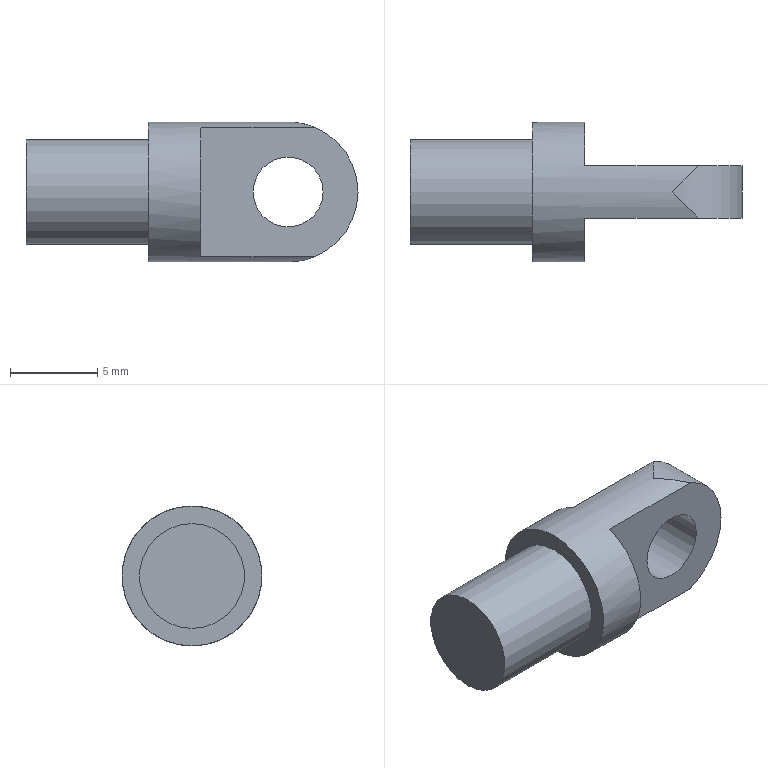Part | NX | features solid 2 | 1 solid | 10 faces | box 19 x 8 x 8 mm | volume 503.106 mm3 | plane 6 | cylinder 4 | commonest cylinder face diameters 8 x2 4 x1 6 x1
STEP:
#1=CARTESIAN_POINT('',(1365.5,900.,-71.));
#2=VERTEX_POINT('',#1);
#3=CARTESIAN_POINT('',(1365.5,900.,-75.));
#4=DIRECTION('',(1.,0.,0.));
#5=DIRECTION('',(0.,0.,1.));
#6=AXIS2_PLACEMENT_3D('',#3,#4,#5);
#7=CIRCLE('',#6,4.);
#8=EDGE_CURVE('',#2,#2,#7,.T.);
#9=ORIENTED_EDGE('',*,*,#8,.T.);
#10=EDGE_LOOP('',(#9));
#11=FACE_BOUND('',#10,.T.);
#12=CARTESIAN_POINT('',(1368.5,898.5,-71.292));
#13=VERTEX_POINT('',#12);
#14=CARTESIAN_POINT('',(1368.5,898.5,-78.708));
#15=VERTEX_POINT('',#14);
#16=CARTESIAN_POINT('',(1368.5,900.,-75.));
#17=DIRECTION('',(1.,0.,0.));
#18=DIRECTION('',(0.,0.,-1.));
#19=AXIS2_PLACEMENT_3D('',#16,#17,#18);
#20=CIRCLE('',#19,4.);
#21=EDGE_CURVE('',#13,#15,#20,.T.);
#22=ORIENTED_EDGE('',*,*,#21,.F.);
#23=CARTESIAN_POINT('',(1375.,898.5,-71.292));
#24=VERTEX_POINT('',#23);
#25=CARTESIAN_POINT('',(1377.5,898.5,-71.292));
#26=DIRECTION('',(-1.,0.,0.));
#27=VECTOR('',#26,1000.);
#28=LINE('',#25,#27);
#29=EDGE_CURVE('',#24,#13,#28,.T.);
#30=ORIENTED_EDGE('',*,*,#29,.F.);
#31=CARTESIAN_POINT('',(1373.5,900.,-71.));
#32=VERTEX_POINT('',#31);
#33=CARTESIAN_POINT('',(1373.5,900.,-75.));
#34=DIRECTION('',(-0.7071,-0.7071,0.));
#35=DIRECTION('',(-0.7071,0.7071,0.));
#36=AXIS2_PLACEMENT_3D('',#33,#34,#35);
#37=ELLIPSE('',#36,5.657,4.);
#38=EDGE_CURVE('',#24,#32,#37,.T.);
#39=ORIENTED_EDGE('',*,*,#38,.T.);
#40=CARTESIAN_POINT('',(1375.,901.5,-71.292));
#41=VERTEX_POINT('',#40);
#42=CARTESIAN_POINT('',(1373.5,900.,-75.));
#43=DIRECTION('',(-0.7071,0.7071,0.));
#44=DIRECTION('',(-0.7071,-0.7071,0.));
#45=AXIS2_PLACEMENT_3D('',#42,#43,#44);
#46=ELLIPSE('',#45,5.657,4.);
#47=EDGE_CURVE('',#32,#41,#46,.T.);
#48=ORIENTED_EDGE('',*,*,#47,.T.);
#49=CARTESIAN_POINT('',(1368.5,901.5,-71.292));
#50=VERTEX_POINT('',#49);
#51=CARTESIAN_POINT('',(1377.5,901.5,-71.292));
#52=DIRECTION('',(-1.,0.,0.));
#53=VECTOR('',#52,1000.);
#54=LINE('',#51,#53);
#55=EDGE_CURVE('',#50,#41,#54,.F.);
#56=ORIENTED_EDGE('',*,*,#55,.F.);
#57=CARTESIAN_POINT('',(1368.5,901.5,-78.708));
#58=VERTEX_POINT('',#57);
#59=CARTESIAN_POINT('',(1368.5,900.,-75.));
#60=DIRECTION('',(1.,0.,0.));
#61=DIRECTION('',(0.,0.,-1.));
#62=AXIS2_PLACEMENT_3D('',#59,#60,#61);
#63=CIRCLE('',#62,4.);
#64=EDGE_CURVE('',#58,#50,#63,.T.);
#65=ORIENTED_EDGE('',*,*,#64,.F.);
#66=CARTESIAN_POINT('',(1375.,901.5,-78.708));
#67=VERTEX_POINT('',#66);
#68=CARTESIAN_POINT('',(1377.5,901.5,-78.708));
#69=DIRECTION('',(-1.,0.,0.));
#70=VECTOR('',#69,1000.);
#71=LINE('',#68,#70);
#72=EDGE_CURVE('',#67,#58,#71,.T.);
#73=ORIENTED_EDGE('',*,*,#72,.F.);
#74=CARTESIAN_POINT('',(1373.5,900.,-79.));
#75=VERTEX_POINT('',#74);
#76=CARTESIAN_POINT('',(1373.5,900.,-75.));
#77=DIRECTION('',(-0.7071,0.7071,0.));
#78=DIRECTION('',(-0.7071,-0.7071,0.));
#79=AXIS2_PLACEMENT_3D('',#76,#77,#78);
#80=ELLIPSE('',#79,5.657,4.);
#81=EDGE_CURVE('',#67,#75,#80,.T.);
#82=ORIENTED_EDGE('',*,*,#81,.T.);
#83=CARTESIAN_POINT('',(1375.,898.5,-78.708));
#84=VERTEX_POINT('',#83);
#85=CARTESIAN_POINT('',(1373.5,900.,-75.));
#86=DIRECTION('',(-0.7071,-0.7071,0.));
#87=DIRECTION('',(-0.7071,0.7071,0.));
#88=AXIS2_PLACEMENT_3D('',#85,#86,#87);
#89=ELLIPSE('',#88,5.657,4.);
#90=EDGE_CURVE('',#75,#84,#89,.T.);
#91=ORIENTED_EDGE('',*,*,#90,.T.);
#92=CARTESIAN_POINT('',(1377.5,898.5,-78.708));
#93=DIRECTION('',(-1.,0.,0.));
#94=VECTOR('',#93,1000.);
#95=LINE('',#92,#94);
#96=EDGE_CURVE('',#15,#84,#95,.F.);
#97=ORIENTED_EDGE('',*,*,#96,.F.);
#98=EDGE_LOOP('',(#22,#30,#39,#48,#56,#65,#73,#82,#91,#97));
#99=FACE_BOUND('',#98,.T.);
#100=CARTESIAN_POINT('',(1377.5,900.,-75.));
#101=DIRECTION('',(-1.,0.,0.));
#102=DIRECTION('',(0.,0.,1.));
#103=AXIS2_PLACEMENT_3D('',#100,#101,#102);
#104=CYLINDRICAL_SURFACE('',#103,4.);
#105=ADVANCED_FACE('',(#11,#99),#104,.T.);
#106=CARTESIAN_POINT('',(1365.5,900.,-78.));
#107=VERTEX_POINT('',#106);
#108=CARTESIAN_POINT('',(1365.5,900.,-75.));
#109=DIRECTION('',(1.,0.,0.));
#110=DIRECTION('',(0.,0.,-1.));
#111=AXIS2_PLACEMENT_3D('',#108,#109,#110);
#112=CIRCLE('',#111,3.);
#113=EDGE_CURVE('',#107,#107,#112,.T.);
#114=ORIENTED_EDGE('',*,*,#113,.T.);
#115=EDGE_LOOP('',(#114));
#116=FACE_BOUND('',#115,.T.);
#117=ORIENTED_EDGE('',*,*,#8,.F.);
#118=EDGE_LOOP('',(#117));
#119=FACE_BOUND('',#118,.T.);
#120=CARTESIAN_POINT('',(1365.5,900.,-75.));
#121=DIRECTION('',(1.,0.,0.));
#122=DIRECTION('',(0.,0.,-1.));
#123=AXIS2_PLACEMENT_3D('',#120,#121,#122);
#124=PLANE('',#123);
#125=ADVANCED_FACE('',(#116,#119),#124,.F.);
#126=CARTESIAN_POINT('',(1373.5,901.5,-75.));
#127=DIRECTION('',(0.,1.,0.));
#128=DIRECTION('',(-1.,0.,0.));
#129=AXIS2_PLACEMENT_3D('',#126,#127,#128);
#130=CIRCLE('',#129,4.);
#131=EDGE_CURVE('',#41,#67,#130,.T.);
#132=ORIENTED_EDGE('',*,*,#131,.F.);
#133=ORIENTED_EDGE('',*,*,#47,.F.);
#134=ORIENTED_EDGE('',*,*,#38,.F.);
#135=CARTESIAN_POINT('',(1373.5,898.5,-75.));
#136=DIRECTION('',(0.,-1.,0.));
#137=DIRECTION('',(1.,0.,0.));
#138=AXIS2_PLACEMENT_3D('',#135,#136,#137);
#139=CIRCLE('',#138,4.);
#140=EDGE_CURVE('',#84,#24,#139,.T.);
#141=ORIENTED_EDGE('',*,*,#140,.F.);
#142=ORIENTED_EDGE('',*,*,#90,.F.);
#143=ORIENTED_EDGE('',*,*,#81,.F.);
#144=EDGE_LOOP('',(#132,#133,#134,#141,#142,#143));
#145=FACE_BOUND('',#144,.T.);
#146=CARTESIAN_POINT('',(1373.5,892.,-75.));
#147=DIRECTION('',(0.,1.,0.));
#148=DIRECTION('',(0.,0.,1.));
#149=AXIS2_PLACEMENT_3D('',#146,#147,#148);
#150=CYLINDRICAL_SURFACE('',#149,4.);
#151=ADVANCED_FACE('',(#145),#150,.T.);
#152=CARTESIAN_POINT('',(1375.5,898.5,-75.));
#153=VERTEX_POINT('',#152);
#154=CARTESIAN_POINT('',(1373.5,898.5,-75.));
#155=DIRECTION('',(0.,-1.,0.));
#156=DIRECTION('',(1.,0.,0.));
#157=AXIS2_PLACEMENT_3D('',#154,#155,#156);
#158=CIRCLE('',#157,2.);
#159=EDGE_CURVE('',#153,#153,#158,.T.);
#160=ORIENTED_EDGE('',*,*,#159,.F.);
#161=EDGE_LOOP('',(#160));
#162=FACE_BOUND('',#161,.T.);
#163=ORIENTED_EDGE('',*,*,#140,.T.);
#164=ORIENTED_EDGE('',*,*,#29,.T.);
#165=CARTESIAN_POINT('',(1368.5,898.5,-70.));
#166=DIRECTION('',(0.,0.,-1.));
#167=VECTOR('',#166,1000.);
#168=LINE('',#165,#167);
#169=EDGE_CURVE('',#13,#15,#168,.T.);
#170=ORIENTED_EDGE('',*,*,#169,.T.);
#171=ORIENTED_EDGE('',*,*,#96,.T.);
#172=EDGE_LOOP('',(#163,#164,#170,#171));
#173=FACE_BOUND('',#172,.T.);
#174=CARTESIAN_POINT('',(1377.5,898.5,-70.));
#175=DIRECTION('',(0.,-1.,0.));
#176=DIRECTION('',(1.,0.,0.));
#177=AXIS2_PLACEMENT_3D('',#174,#175,#176);
#178=PLANE('',#177);
#179=ADVANCED_FACE('',(#162,#173),#178,.T.);
#180=ORIENTED_EDGE('',*,*,#169,.F.);
#181=ORIENTED_EDGE('',*,*,#21,.T.);
#182=EDGE_LOOP('',(#180,#181));
#183=FACE_BOUND('',#182,.T.);
#184=CARTESIAN_POINT('',(1368.5,898.5,-70.));
#185=DIRECTION('',(1.,0.,0.));
#186=DIRECTION('',(0.,0.,-1.));
#187=AXIS2_PLACEMENT_3D('',#184,#185,#186);
#188=PLANE('',#187);
#189=ADVANCED_FACE('',(#183),#188,.T.);
#190=CARTESIAN_POINT('',(1368.5,901.5,-70.));
#191=DIRECTION('',(0.,0.,-1.));
#192=VECTOR('',#191,1000.);
#193=LINE('',#190,#192);
#194=EDGE_CURVE('',#50,#58,#193,.T.);
#195=ORIENTED_EDGE('',*,*,#194,.T.);
#196=ORIENTED_EDGE('',*,*,#64,.T.);
#197=EDGE_LOOP('',(#195,#196));
#198=FACE_BOUND('',#197,.T.);
#199=CARTESIAN_POINT('',(1368.5,904.,-70.));
#200=DIRECTION('',(1.,0.,0.));
#201=DIRECTION('',(0.,0.,-1.));
#202=AXIS2_PLACEMENT_3D('',#199,#200,#201);
#203=PLANE('',#202);
#204=ADVANCED_FACE('',(#198),#203,.T.);
#205=CARTESIAN_POINT('',(1371.5,901.5,-75.));
#206=VERTEX_POINT('',#205);
#207=CARTESIAN_POINT('',(1373.5,901.5,-75.));
#208=DIRECTION('',(0.,1.,0.));
#209=DIRECTION('',(-1.,0.,0.));
#210=AXIS2_PLACEMENT_3D('',#207,#208,#209);
#211=CIRCLE('',#210,2.);
#212=EDGE_CURVE('',#206,#206,#211,.T.);
#213=ORIENTED_EDGE('',*,*,#212,.F.);
#214=EDGE_LOOP('',(#213));
#215=FACE_BOUND('',#214,.T.);
#216=ORIENTED_EDGE('',*,*,#131,.T.);
#217=ORIENTED_EDGE('',*,*,#72,.T.);
#218=ORIENTED_EDGE('',*,*,#194,.F.);
#219=ORIENTED_EDGE('',*,*,#55,.T.);
#220=EDGE_LOOP('',(#216,#217,#218,#219));
#221=FACE_BOUND('',#220,.T.);
#222=CARTESIAN_POINT('',(1368.5,901.5,-70.));
#223=DIRECTION('',(0.,1.,0.));
#224=DIRECTION('',(-1.,0.,0.));
#225=AXIS2_PLACEMENT_3D('',#222,#223,#224);
#226=PLANE('',#225);
#227=ADVANCED_FACE('',(#215,#221),#226,.T.);
#228=ORIENTED_EDGE('',*,*,#212,.T.);
#229=EDGE_LOOP('',(#228));
#230=FACE_BOUND('',#229,.T.);
#231=ORIENTED_EDGE('',*,*,#159,.T.);
#232=EDGE_LOOP('',(#231));
#233=FACE_BOUND('',#232,.T.);
#234=CARTESIAN_POINT('',(1373.5,892.,-75.));
#235=DIRECTION('',(0.,1.,0.));
#236=DIRECTION('',(0.,0.,1.));
#237=AXIS2_PLACEMENT_3D('',#234,#235,#236);
#238=CYLINDRICAL_SURFACE('',#237,2.);
#239=ADVANCED_FACE('',(#230,#233),#238,.F.);
#240=CARTESIAN_POINT('',(1358.5,900.,-72.));
#241=VERTEX_POINT('',#240);
#242=CARTESIAN_POINT('',(1358.5,900.,-75.));
#243=DIRECTION('',(1.,0.,0.));
#244=DIRECTION('',(0.,0.,1.));
#245=AXIS2_PLACEMENT_3D('',#242,#243,#244);
#246=CIRCLE('',#245,3.);
#247=EDGE_CURVE('',#241,#241,#246,.T.);
#248=ORIENTED_EDGE('',*,*,#247,.T.);
#249=EDGE_LOOP('',(#248));
#250=FACE_BOUND('',#249,.T.);
#251=ORIENTED_EDGE('',*,*,#113,.F.);
#252=EDGE_LOOP('',(#251));
#253=FACE_BOUND('',#252,.T.);
#254=CARTESIAN_POINT('',(1358.5,900.,-75.));
#255=DIRECTION('',(1.,0.,0.));
#256=DIRECTION('',(0.,0.,-1.));
#257=AXIS2_PLACEMENT_3D('',#254,#255,#256);
#258=CYLINDRICAL_SURFACE('',#257,3.);
#259=ADVANCED_FACE('',(#250,#253),#258,.T.);
#260=ORIENTED_EDGE('',*,*,#247,.F.);
#261=EDGE_LOOP('',(#260));
#262=FACE_BOUND('',#261,.T.);
#263=CARTESIAN_POINT('',(1358.5,900.,-75.));
#264=DIRECTION('',(1.,0.,0.));
#265=DIRECTION('',(0.,0.,-1.));
#266=AXIS2_PLACEMENT_3D('',#263,#264,#265);
#267=PLANE('',#266);
#268=ADVANCED_FACE('',(#262),#267,.F.);
#269=CLOSED_SHELL('',(#105,#125,#151,#179,#189,#204,#227,#239,#259,#268));
#270=MANIFOLD_SOLID_BREP('',#269);
#271=(LENGTH_UNIT()NAMED_UNIT(*)SI_UNIT(.MILLI.,.METRE.));
#272=UNCERTAINTY_MEASURE_WITH_UNIT(LENGTH_MEASURE(0.00001),#271,'','');
#273=(NAMED_UNIT(*)PLANE_ANGLE_UNIT()SI_UNIT($,.RADIAN.));
#274=(NAMED_UNIT(*)SI_UNIT($,.STERADIAN.)SOLID_ANGLE_UNIT());
#275=(GEOMETRIC_REPRESENTATION_CONTEXT(3)GLOBAL_UNCERTAINTY_ASSIGNED_CONTEXT((#272))GLOBAL_UNIT_ASSIGNED_CONTEXT((#271,#273,#274))REPRESENTATION_CONTEXT('',''));
#276=ADVANCED_BREP_SHAPE_REPRESENTATION('',(#270),#275);